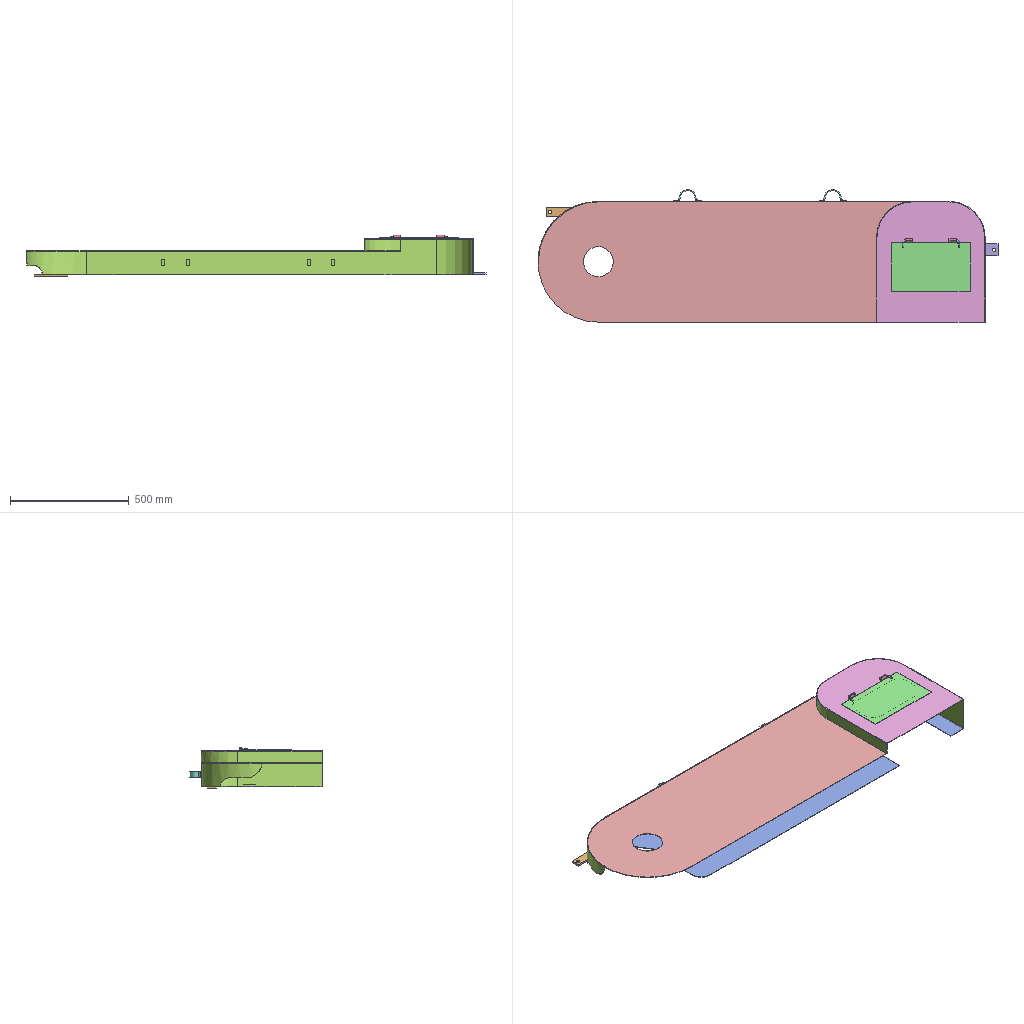Assembly | SolidWorks | 10 different items | 13 placed | box 1933 x 557 x 174 mm
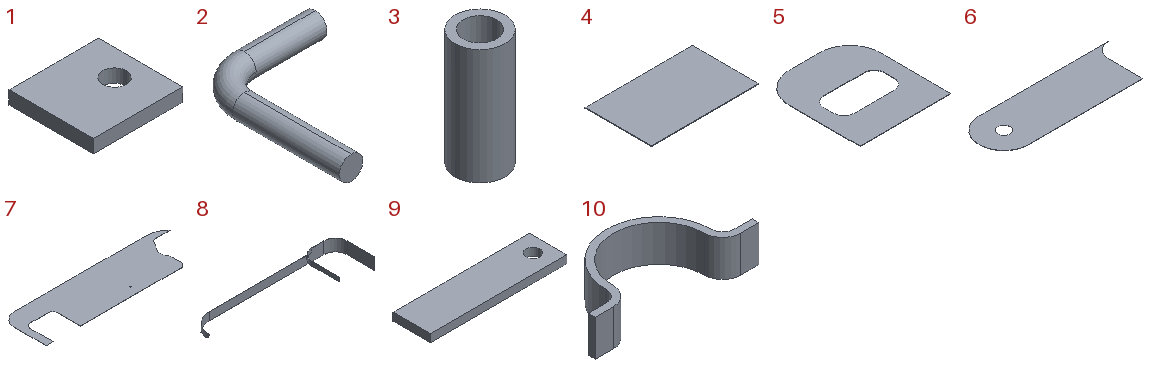Parts list (item | quantity | size | volume | features):
1 | x1 | 53.848 x 50.8 x 8 mm | 20604 mm3 | features Extrusion 1
2 | x2 | 31.75 x 41.402 x 6.35 mm | 1986 mm3 | features Sweep 1
3 | x2 | 13.7 x 13.7 x 31.75 mm | 2561 mm3 | features Extrusion 1
4 | x1 | 330.2 x 203.2 x 2 mm | 134193 mm3 | features Extrusion 1
5 | x1 | 457.2 x 508 x 2 mm | 356105 mm3 | features Extrusion 1
6 | x1 | 1575 x 508 x 2 mm | 1374411 mm3 | features Extrusion 1
7 | x1 | 1812 x 508 x 2 mm | 1419003 mm3 | features Extrusion 1
8 | x1 | 1880 x 508 x 152.4 mm | 621350 mm3 | features ICE 2, Extrusion 1
9 | x1 | 139.7 x 38.1 x 8 mm | 41300 mm3 | features Extrusion 1
10 | x2 | 114.3 x 49.213 x 25.4 mm | 19965 mm3 | features Extrusion 1, RefAxis 1
Mates (type | each side: item.copy, entity, surface, feature):
Coincident | 6.1 plane | assembly plane | 2 times
Coincident | 7.1 plane | assembly plane | 2 times
Symmetric | 6.1 face plane Boss-Extrude1 | 7.1 face plane Boss-Extrude1 | assembly plane
Coincident | 8.1 plane | assembly plane | 2 times
Coincident | 7.1 face plane Boss-Extrude1 | 8.1 face plane Boss-Extrude1
Coincident | 6.1 face plane Boss-Extrude1 | 8.1 face plane Boss-Extrude1
Concentric | 7.1 face cylinder Boss-Extrude1 | 5.1 face cylinder Boss-Extrude1 | 2 times
Coincident | 8.1 face plane Boss-Extrude2 | 5.1 face plane Boss-Extrude1
Coincident | 8.1 face plane Boss-Extrude1 | 10.1 face plane Boss-Extrude1
Coincident | 10.1 plane | assembly plane
Coincident | 7.1 face plane Boss-Extrude1 | 9.1 face plane Boss-Extrude1
DistanceDim | 9.1 plane | assembly plane | 2 times
Coincident | 7.1 face plane Boss-Extrude1 | 1.1 face plane Boss-Extrude1
Coincident | 8.1 face plane Boss-Extrude1 | 1.1 face plane Boss-Extrude1
DistanceDim | 1.1 plane | 8.1 face plane Boss-Extrude1
Symmetric | 5.1 face plane Boss-Extrude1 | 5.1 face plane Boss-Extrude1 | 4.1 plane
Tangent | 5.1 face plane Boss-Extrude1 | 3.1 face cylinder Boss-Extrude1
DistanceDim | 3.1 plane | assembly plane
Concentric | 2.1 face cylinder Sweep1 | 3.1 face cylinder Boss-Extrude1
Coincident | 3.1 face plane Boss-Extrude1 | 2.1 edge
Tangent | 4.1 face plane Boss-Extrude1 | 2.1 face cylinder Sweep1
DistanceDim | 3.1 face plane Boss-Extrude1 | 3.2 face plane Boss-Extrude1
DistanceDim | 4.1 face plane Boss-Extrude1 | 2.1 face plane Sweep1
DistanceDim | 10.2 face plane Boss-Extrude1 | 8.1 face plane Boss-Extrude1